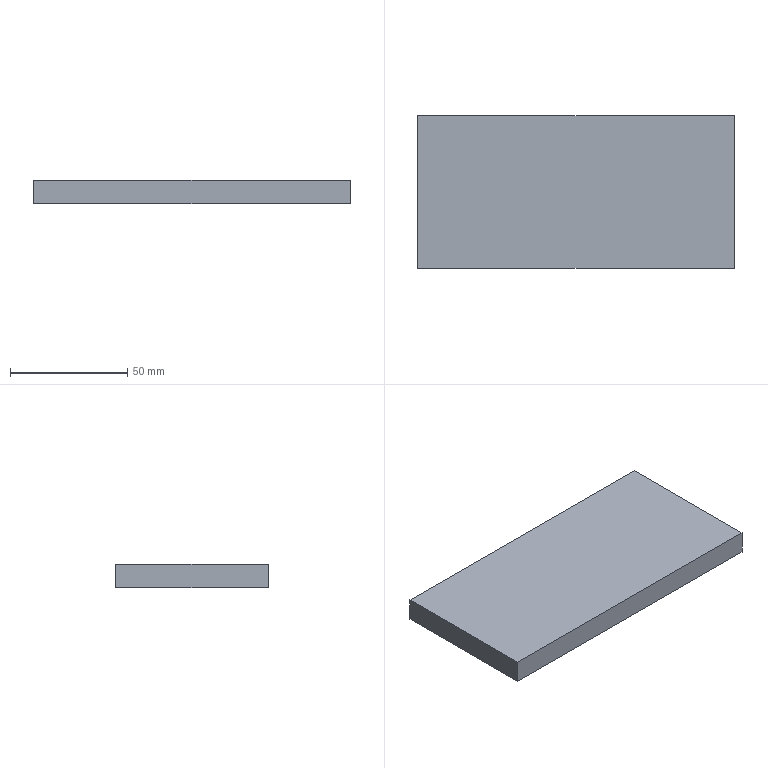Part | STEP file | Frame Screw Feeder | 1 solid | 6 faces | box 135 x 65 x 10 mm | volume 87750 mm3 | plane 6
STEP:
#1=CARTESIAN_POINT('',(146.928,1106.2,36.326));
#2=VERTEX_POINT('',#1);
#3=CARTESIAN_POINT('',(11.928,1106.2,36.326));
#4=VERTEX_POINT('',#3);
#5=CARTESIAN_POINT('',(146.928,1106.2,36.326));
#6=DIRECTION('',(-1.,0.,0.));
#7=VECTOR('',#6,10.);
#8=LINE('',#5,#7);
#9=EDGE_CURVE('',#2,#4,#8,.T.);
#10=ORIENTED_EDGE('',*,*,#9,.T.);
#11=CARTESIAN_POINT('',(11.928,1106.2,46.326));
#12=VERTEX_POINT('',#11);
#13=CARTESIAN_POINT('',(11.928,1106.2,36.326));
#14=DIRECTION('',(0.,0.,1.));
#15=VECTOR('',#14,10.);
#16=LINE('',#13,#15);
#17=EDGE_CURVE('',#4,#12,#16,.T.);
#18=ORIENTED_EDGE('',*,*,#17,.T.);
#19=CARTESIAN_POINT('',(146.928,1106.2,46.326));
#20=VERTEX_POINT('',#19);
#21=CARTESIAN_POINT('',(146.928,1106.2,46.326));
#22=DIRECTION('',(-1.,0.,0.));
#23=VECTOR('',#22,10.);
#24=LINE('',#21,#23);
#25=EDGE_CURVE('',#20,#12,#24,.T.);
#26=ORIENTED_EDGE('',*,*,#25,.F.);
#27=CARTESIAN_POINT('',(146.928,1106.2,36.326));
#28=DIRECTION('',(0.,0.,1.));
#29=VECTOR('',#28,10.);
#30=LINE('',#27,#29);
#31=EDGE_CURVE('',#2,#20,#30,.T.);
#32=ORIENTED_EDGE('',*,*,#31,.F.);
#33=EDGE_LOOP('',(#10,#18,#26,#32));
#34=FACE_OUTER_BOUND('',#33,.T.);
#35=CARTESIAN_POINT('',(146.928,1106.2,36.326));
#36=DIRECTION('',(0.,1.,0.));
#37=DIRECTION('',(-1.,0.,0.));
#38=AXIS2_PLACEMENT_3D('',#35,#36,#37);
#39=PLANE('',#38);
#40=ADVANCED_FACE('',(#34),#39,.T.);
#41=CARTESIAN_POINT('',(146.928,1041.2,36.326));
#42=VERTEX_POINT('',#41);
#43=CARTESIAN_POINT('',(146.928,1041.2,36.326));
#44=DIRECTION('',(0.,1.,0.));
#45=VECTOR('',#44,10.);
#46=LINE('',#43,#45);
#47=EDGE_CURVE('',#42,#2,#46,.T.);
#48=ORIENTED_EDGE('',*,*,#47,.T.);
#49=ORIENTED_EDGE('',*,*,#31,.T.);
#50=CARTESIAN_POINT('',(146.928,1041.2,46.326));
#51=VERTEX_POINT('',#50);
#52=CARTESIAN_POINT('',(146.928,1041.2,46.326));
#53=DIRECTION('',(0.,1.,0.));
#54=VECTOR('',#53,10.);
#55=LINE('',#52,#54);
#56=EDGE_CURVE('',#51,#20,#55,.T.);
#57=ORIENTED_EDGE('',*,*,#56,.F.);
#58=CARTESIAN_POINT('',(146.928,1041.2,36.326));
#59=DIRECTION('',(0.,0.,1.));
#60=VECTOR('',#59,10.);
#61=LINE('',#58,#60);
#62=EDGE_CURVE('',#42,#51,#61,.T.);
#63=ORIENTED_EDGE('',*,*,#62,.F.);
#64=EDGE_LOOP('',(#48,#49,#57,#63));
#65=FACE_OUTER_BOUND('',#64,.T.);
#66=CARTESIAN_POINT('',(146.928,1041.2,36.326));
#67=DIRECTION('',(1.,0.,0.));
#68=DIRECTION('',(0.,1.,0.));
#69=AXIS2_PLACEMENT_3D('',#66,#67,#68);
#70=PLANE('',#69);
#71=ADVANCED_FACE('',(#65),#70,.T.);
#72=CARTESIAN_POINT('',(11.928,1041.2,36.326));
#73=VERTEX_POINT('',#72);
#74=CARTESIAN_POINT('',(11.928,1041.2,36.326));
#75=DIRECTION('',(1.,0.,0.));
#76=VECTOR('',#75,10.);
#77=LINE('',#74,#76);
#78=EDGE_CURVE('',#73,#42,#77,.T.);
#79=ORIENTED_EDGE('',*,*,#78,.T.);
#80=ORIENTED_EDGE('',*,*,#62,.T.);
#81=CARTESIAN_POINT('',(11.928,1041.2,46.326));
#82=VERTEX_POINT('',#81);
#83=CARTESIAN_POINT('',(11.928,1041.2,46.326));
#84=DIRECTION('',(1.,0.,0.));
#85=VECTOR('',#84,10.);
#86=LINE('',#83,#85);
#87=EDGE_CURVE('',#82,#51,#86,.T.);
#88=ORIENTED_EDGE('',*,*,#87,.F.);
#89=CARTESIAN_POINT('',(11.928,1041.2,36.326));
#90=DIRECTION('',(0.,0.,1.));
#91=VECTOR('',#90,10.);
#92=LINE('',#89,#91);
#93=EDGE_CURVE('',#73,#82,#92,.T.);
#94=ORIENTED_EDGE('',*,*,#93,.F.);
#95=EDGE_LOOP('',(#79,#80,#88,#94));
#96=FACE_OUTER_BOUND('',#95,.T.);
#97=CARTESIAN_POINT('',(11.928,1041.2,36.326));
#98=DIRECTION('',(0.,-1.,0.));
#99=DIRECTION('',(1.,0.,0.));
#100=AXIS2_PLACEMENT_3D('',#97,#98,#99);
#101=PLANE('',#100);
#102=ADVANCED_FACE('',(#96),#101,.T.);
#103=CARTESIAN_POINT('',(11.928,1106.2,36.326));
#104=DIRECTION('',(0.,-1.,0.));
#105=VECTOR('',#104,10.);
#106=LINE('',#103,#105);
#107=EDGE_CURVE('',#4,#73,#106,.T.);
#108=ORIENTED_EDGE('',*,*,#107,.T.);
#109=ORIENTED_EDGE('',*,*,#93,.T.);
#110=CARTESIAN_POINT('',(11.928,1106.2,46.326));
#111=DIRECTION('',(0.,-1.,0.));
#112=VECTOR('',#111,10.);
#113=LINE('',#110,#112);
#114=EDGE_CURVE('',#12,#82,#113,.T.);
#115=ORIENTED_EDGE('',*,*,#114,.F.);
#116=ORIENTED_EDGE('',*,*,#17,.F.);
#117=EDGE_LOOP('',(#108,#109,#115,#116));
#118=FACE_OUTER_BOUND('',#117,.T.);
#119=CARTESIAN_POINT('',(11.928,1106.2,36.326));
#120=DIRECTION('',(-1.,0.,0.));
#121=DIRECTION('',(0.,-1.,0.));
#122=AXIS2_PLACEMENT_3D('',#119,#120,#121);
#123=PLANE('',#122);
#124=ADVANCED_FACE('',(#118),#123,.T.);
#125=ORIENTED_EDGE('',*,*,#114,.T.);
#126=ORIENTED_EDGE('',*,*,#87,.T.);
#127=ORIENTED_EDGE('',*,*,#56,.T.);
#128=ORIENTED_EDGE('',*,*,#25,.T.);
#129=EDGE_LOOP('',(#125,#126,#127,#128));
#130=FACE_OUTER_BOUND('',#129,.T.);
#131=CARTESIAN_POINT('',(79.428,1073.7,46.326));
#132=DIRECTION('',(0.,0.,1.));
#133=DIRECTION('',(1.,0.,0.));
#134=AXIS2_PLACEMENT_3D('',#131,#132,#133);
#135=PLANE('',#134);
#136=ADVANCED_FACE('',(#130),#135,.T.);
#137=ORIENTED_EDGE('',*,*,#107,.F.);
#138=ORIENTED_EDGE('',*,*,#9,.F.);
#139=ORIENTED_EDGE('',*,*,#47,.F.);
#140=ORIENTED_EDGE('',*,*,#78,.F.);
#141=EDGE_LOOP('',(#137,#138,#139,#140));
#142=FACE_OUTER_BOUND('',#141,.T.);
#143=CARTESIAN_POINT('',(79.428,1073.7,36.326));
#144=DIRECTION('',(0.,0.,1.));
#145=DIRECTION('',(1.,0.,0.));
#146=AXIS2_PLACEMENT_3D('',#143,#144,#145);
#147=PLANE('',#146);
#148=ADVANCED_FACE('',(#142),#147,.F.);
#149=CLOSED_SHELL('',(#40,#71,#102,#124,#136,#148));
#150=MANIFOLD_SOLID_BREP('',#149);
#151=(LENGTH_UNIT()NAMED_UNIT(*)SI_UNIT(.MILLI.,.METRE.));
#152=UNCERTAINTY_MEASURE_WITH_UNIT(LENGTH_MEASURE(0.01),#151,'','');
#153=(NAMED_UNIT(*)PLANE_ANGLE_UNIT()SI_UNIT($,.RADIAN.));
#154=(NAMED_UNIT(*)SI_UNIT($,.STERADIAN.)SOLID_ANGLE_UNIT());
#155=(GEOMETRIC_REPRESENTATION_CONTEXT(3)GLOBAL_UNCERTAINTY_ASSIGNED_CONTEXT((#152))GLOBAL_UNIT_ASSIGNED_CONTEXT((#151,#153,#154))REPRESENTATION_CONTEXT('',''));
#156=ADVANCED_BREP_SHAPE_REPRESENTATION('',(#150),#155);